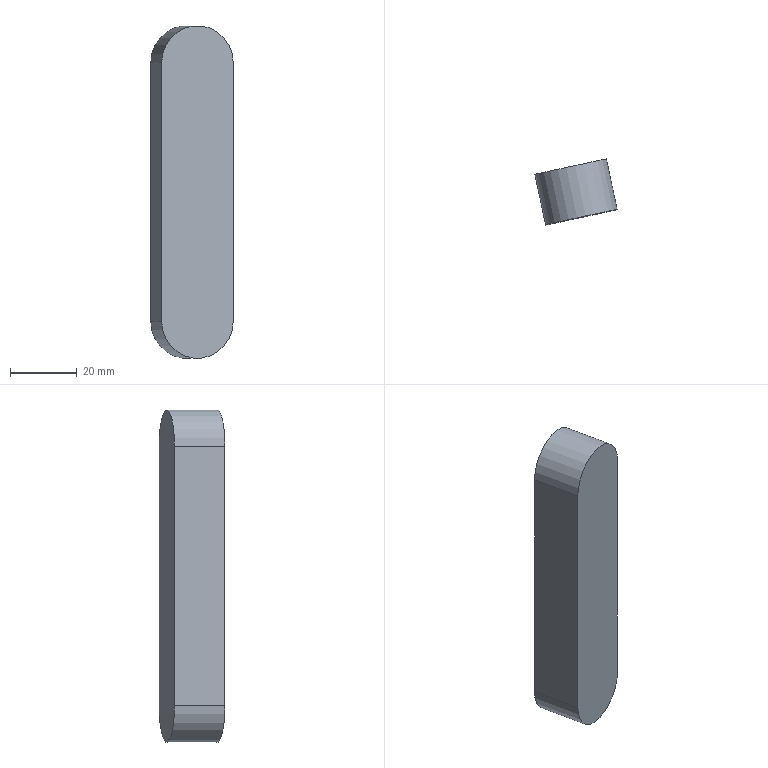Part | SolidWorks | features BaseBody 1 | 1 solid | 6 faces | box 24.773 x 19.79 x 100 mm | volume 32490 mm3 | plane 4 | cylinder 2 | commonest cylinder face diameters 22 x2
STEP:
#1=CARTESIAN_POINT('',(-741.788,459.923,828.107));
#2=VERTEX_POINT('',#1);
#3=CARTESIAN_POINT('',(-763.294,455.284,828.107));
#4=VERTEX_POINT('',#3);
#5=CARTESIAN_POINT('',(-752.541,457.604,828.107));
#6=DIRECTION('',(0.2108,-0.9775,0.));
#7=DIRECTION('',(-0.9775,-0.2108,0.));
#8=AXIS2_PLACEMENT_3D('',#5,#6,#7);
#9=CIRCLE('',#8,11.);
#10=EDGE_CURVE('',#2,#4,#9,.T.);
#11=ORIENTED_EDGE('',*,*,#10,.T.);
#12=CARTESIAN_POINT('',(-763.294,455.284,750.107));
#13=VERTEX_POINT('',#12);
#14=CARTESIAN_POINT('',(-763.294,455.284,739.107));
#15=DIRECTION('',(0.,0.,1.));
#16=VECTOR('',#15,1000.);
#17=LINE('',#14,#16);
#18=EDGE_CURVE('',#13,#4,#17,.T.);
#19=ORIENTED_EDGE('',*,*,#18,.F.);
#20=CARTESIAN_POINT('',(-741.788,459.923,750.107));
#21=VERTEX_POINT('',#20);
#22=CARTESIAN_POINT('',(-752.541,457.604,750.107));
#23=DIRECTION('',(0.2108,-0.9775,0.));
#24=DIRECTION('',(-0.9775,-0.2108,0.));
#25=AXIS2_PLACEMENT_3D('',#22,#23,#24);
#26=CIRCLE('',#25,11.);
#27=EDGE_CURVE('',#13,#21,#26,.T.);
#28=ORIENTED_EDGE('',*,*,#27,.T.);
#29=CARTESIAN_POINT('',(-741.788,459.923,739.107));
#30=DIRECTION('',(0.,0.,1.));
#31=VECTOR('',#30,1000.);
#32=LINE('',#29,#31);
#33=EDGE_CURVE('',#21,#2,#32,.T.);
#34=ORIENTED_EDGE('',*,*,#33,.T.);
#35=EDGE_LOOP('',(#11,#19,#28,#34));
#36=FACE_OUTER_BOUND('',#35,.T.);
#37=CARTESIAN_POINT('',(-757.428,456.549,739.107));
#38=DIRECTION('',(-0.2108,0.9775,0.));
#39=DIRECTION('',(0.,0.,1.));
#40=AXIS2_PLACEMENT_3D('',#37,#38,#39);
#41=PLANE('',#40);
#42=ADVANCED_FACE('',(#36),#41,.F.);
#43=CARTESIAN_POINT('',(-745.056,475.074,828.107));
#44=VERTEX_POINT('',#43);
#45=CARTESIAN_POINT('',(-766.562,470.436,828.107));
#46=VERTEX_POINT('',#45);
#47=CARTESIAN_POINT('',(-755.809,472.755,828.107));
#48=DIRECTION('',(0.2108,-0.9775,0.));
#49=DIRECTION('',(-0.9775,-0.2108,0.));
#50=AXIS2_PLACEMENT_3D('',#47,#48,#49);
#51=CIRCLE('',#50,11.);
#52=EDGE_CURVE('',#44,#46,#51,.T.);
#53=ORIENTED_EDGE('',*,*,#52,.F.);
#54=CARTESIAN_POINT('',(-745.056,475.074,750.107));
#55=VERTEX_POINT('',#54);
#56=CARTESIAN_POINT('',(-745.056,475.074,739.107));
#57=DIRECTION('',(0.,0.,1.));
#58=VECTOR('',#57,1000.);
#59=LINE('',#56,#58);
#60=EDGE_CURVE('',#55,#44,#59,.T.);
#61=ORIENTED_EDGE('',*,*,#60,.F.);
#62=CARTESIAN_POINT('',(-766.562,470.436,750.107));
#63=VERTEX_POINT('',#62);
#64=CARTESIAN_POINT('',(-755.809,472.755,750.107));
#65=DIRECTION('',(0.2108,-0.9775,0.));
#66=DIRECTION('',(-0.9775,-0.2108,0.));
#67=AXIS2_PLACEMENT_3D('',#64,#65,#66);
#68=CIRCLE('',#67,11.);
#69=EDGE_CURVE('',#63,#55,#68,.T.);
#70=ORIENTED_EDGE('',*,*,#69,.F.);
#71=CARTESIAN_POINT('',(-766.562,470.436,739.107));
#72=DIRECTION('',(0.,0.,1.));
#73=VECTOR('',#72,1000.);
#74=LINE('',#71,#73);
#75=EDGE_CURVE('',#63,#46,#74,.T.);
#76=ORIENTED_EDGE('',*,*,#75,.T.);
#77=EDGE_LOOP('',(#53,#61,#70,#76));
#78=FACE_OUTER_BOUND('',#77,.T.);
#79=CARTESIAN_POINT('',(-760.696,471.701,739.107));
#80=DIRECTION('',(-0.2108,0.9775,0.));
#81=DIRECTION('',(0.,0.,1.));
#82=AXIS2_PLACEMENT_3D('',#79,#80,#81);
#83=PLANE('',#82);
#84=ADVANCED_FACE('',(#78),#83,.T.);
#85=ORIENTED_EDGE('',*,*,#33,.F.);
#86=CARTESIAN_POINT('',(-745.056,475.074,750.107));
#87=DIRECTION('',(0.2108,-0.9775,0.));
#88=VECTOR('',#87,1000.);
#89=LINE('',#86,#88);
#90=EDGE_CURVE('',#55,#21,#89,.T.);
#91=ORIENTED_EDGE('',*,*,#90,.F.);
#92=ORIENTED_EDGE('',*,*,#60,.T.);
#93=CARTESIAN_POINT('',(-745.056,475.074,828.107));
#94=DIRECTION('',(0.2108,-0.9775,0.));
#95=VECTOR('',#94,1000.);
#96=LINE('',#93,#95);
#97=EDGE_CURVE('',#44,#2,#96,.T.);
#98=ORIENTED_EDGE('',*,*,#97,.T.);
#99=EDGE_LOOP('',(#85,#91,#92,#98));
#100=FACE_OUTER_BOUND('',#99,.T.);
#101=CARTESIAN_POINT('',(-745.056,475.074,739.107));
#102=DIRECTION('',(0.9775,0.2108,0.));
#103=DIRECTION('',(0.,0.,-1.));
#104=AXIS2_PLACEMENT_3D('',#101,#102,#103);
#105=PLANE('',#104);
#106=ADVANCED_FACE('',(#100),#105,.T.);
#107=ORIENTED_EDGE('',*,*,#27,.F.);
#108=CARTESIAN_POINT('',(-766.562,470.436,750.107));
#109=DIRECTION('',(0.2108,-0.9775,0.));
#110=VECTOR('',#109,1000.);
#111=LINE('',#108,#110);
#112=EDGE_CURVE('',#63,#13,#111,.T.);
#113=ORIENTED_EDGE('',*,*,#112,.F.);
#114=ORIENTED_EDGE('',*,*,#69,.T.);
#115=ORIENTED_EDGE('',*,*,#90,.T.);
#116=EDGE_LOOP('',(#107,#113,#114,#115));
#117=FACE_OUTER_BOUND('',#116,.T.);
#118=CARTESIAN_POINT('',(-755.809,472.755,750.107));
#119=DIRECTION('',(0.2108,-0.9775,0.));
#120=DIRECTION('',(0.9775,0.2108,0.));
#121=AXIS2_PLACEMENT_3D('',#118,#119,#120);
#122=CYLINDRICAL_SURFACE('',#121,11.);
#123=ADVANCED_FACE('',(#117),#122,.T.);
#124=ORIENTED_EDGE('',*,*,#18,.T.);
#125=CARTESIAN_POINT('',(-766.562,470.436,828.107));
#126=DIRECTION('',(0.2108,-0.9775,0.));
#127=VECTOR('',#126,1000.);
#128=LINE('',#125,#127);
#129=EDGE_CURVE('',#46,#4,#128,.T.);
#130=ORIENTED_EDGE('',*,*,#129,.F.);
#131=ORIENTED_EDGE('',*,*,#75,.F.);
#132=ORIENTED_EDGE('',*,*,#112,.T.);
#133=EDGE_LOOP('',(#124,#130,#131,#132));
#134=FACE_OUTER_BOUND('',#133,.T.);
#135=CARTESIAN_POINT('',(-766.562,470.436,739.107));
#136=DIRECTION('',(0.9775,0.2108,0.));
#137=DIRECTION('',(0.,0.,-1.));
#138=AXIS2_PLACEMENT_3D('',#135,#136,#137);
#139=PLANE('',#138);
#140=ADVANCED_FACE('',(#134),#139,.F.);
#141=ORIENTED_EDGE('',*,*,#10,.F.);
#142=ORIENTED_EDGE('',*,*,#97,.F.);
#143=ORIENTED_EDGE('',*,*,#52,.T.);
#144=ORIENTED_EDGE('',*,*,#129,.T.);
#145=EDGE_LOOP('',(#141,#142,#143,#144));
#146=FACE_OUTER_BOUND('',#145,.T.);
#147=CARTESIAN_POINT('',(-755.809,472.755,828.107));
#148=DIRECTION('',(0.2108,-0.9775,0.));
#149=DIRECTION('',(0.9775,0.2108,0.));
#150=AXIS2_PLACEMENT_3D('',#147,#148,#149);
#151=CYLINDRICAL_SURFACE('',#150,11.);
#152=ADVANCED_FACE('',(#146),#151,.T.);
#153=CLOSED_SHELL('',(#42,#84,#106,#123,#140,#152));
#154=MANIFOLD_SOLID_BREP('',#153);
#155=CARTESIAN_POINT('',(0.,0.,0.));
#156=DIRECTION('',(0.,0.,1.));
#157=DIRECTION('',(1.,0.,0.));
#158=AXIS2_PLACEMENT_3D('',#155,#156,#157);
#159=(LENGTH_UNIT()NAMED_UNIT(*)SI_UNIT(.MILLI.,.METRE.));
#160=UNCERTAINTY_MEASURE_WITH_UNIT(LENGTH_MEASURE(0.00001),#159,'','');
#161=(NAMED_UNIT(*)PLANE_ANGLE_UNIT()SI_UNIT($,.RADIAN.));
#162=(NAMED_UNIT(*)SI_UNIT($,.STERADIAN.)SOLID_ANGLE_UNIT());
#163=(GEOMETRIC_REPRESENTATION_CONTEXT(3)GLOBAL_UNCERTAINTY_ASSIGNED_CONTEXT((#160))GLOBAL_UNIT_ASSIGNED_CONTEXT((#159,#161,#162))REPRESENTATION_CONTEXT('',''));
#164=ADVANCED_BREP_SHAPE_REPRESENTATION('',(#154,#158),#163);